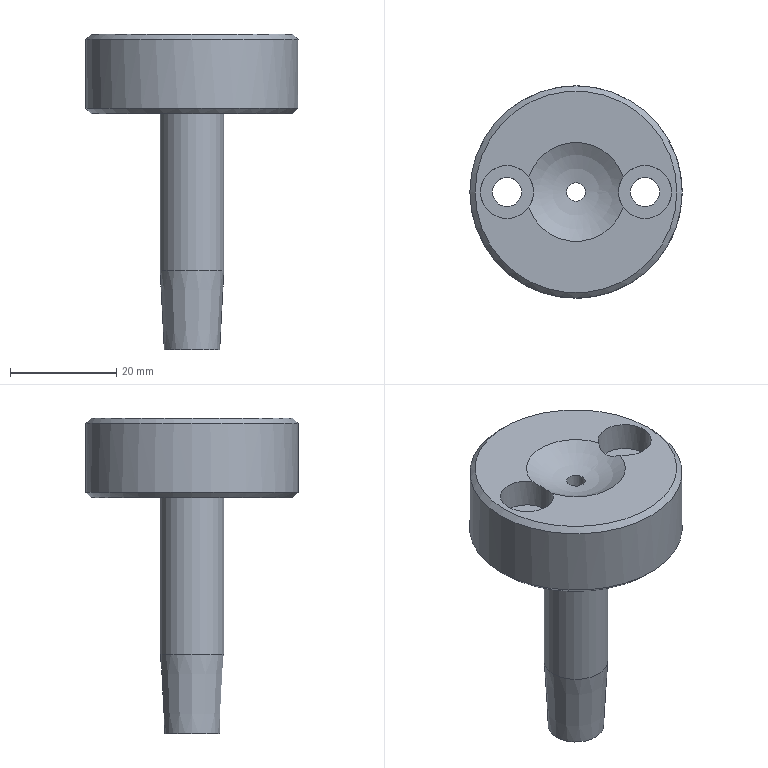Part | STEP file | lll_id154_x_t | 1 solid | 16 faces | box 40 x 40 x 59.5 mm | volume 20901 mm3 | cylinder 6 | plane 5 | cone 4 | sphere 1 | commonest cylinder face diameters 5.5 x2 10 x2 12 x1 40 x1
STEP:
#1=CARTESIAN_POINT('',(-5.214,0.,68.));
#2=VERTEX_POINT('',#1);
#3=CARTESIAN_POINT('',(0.,0.,68.));
#4=DIRECTION('',(0.,0.,1.));
#5=DIRECTION('',(-1.,0.,0.));
#6=AXIS2_PLACEMENT_3D('',#3,#4,#5);
#7=CIRCLE('',#6,5.214);
#8=EDGE_CURVE('',#2,#2,#7,.T.);
#9=ORIENTED_EDGE('',*,*,#8,.F.);
#10=EDGE_LOOP('',(#9));
#11=FACE_BOUND('',#10,.T.);
#12=CARTESIAN_POINT('',(-2.738,0.,68.));
#13=VERTEX_POINT('',#12);
#14=CARTESIAN_POINT('',(0.,0.,68.));
#15=DIRECTION('',(0.,0.,1.));
#16=DIRECTION('',(-1.,0.,0.));
#17=AXIS2_PLACEMENT_3D('',#14,#15,#16);
#18=CIRCLE('',#17,2.738);
#19=EDGE_CURVE('',#13,#13,#18,.T.);
#20=ORIENTED_EDGE('',*,*,#19,.T.);
#21=EDGE_LOOP('',(#20));
#22=FACE_BOUND('',#21,.T.);
#23=CARTESIAN_POINT('',(0.,0.,68.));
#24=DIRECTION('',(0.,0.,-1.));
#25=DIRECTION('',(-1.,0.,0.));
#26=AXIS2_PLACEMENT_3D('',#23,#24,#25);
#27=PLANE('',#26);
#28=ADVANCED_FACE('',(#11,#22),#27,.T.);
#29=CARTESIAN_POINT('',(-19.,0.,112.5));
#30=VERTEX_POINT('',#29);
#31=CARTESIAN_POINT('',(0.,0.,112.5));
#32=DIRECTION('',(0.,0.,-1.));
#33=DIRECTION('',(-1.,0.,0.));
#34=AXIS2_PLACEMENT_3D('',#31,#32,#33);
#35=CIRCLE('',#34,19.);
#36=EDGE_CURVE('',#30,#30,#35,.T.);
#37=ORIENTED_EDGE('',*,*,#36,.T.);
#38=EDGE_LOOP('',(#37));
#39=FACE_BOUND('',#38,.T.);
#40=CARTESIAN_POINT('',(-15.75,0.,112.5));
#41=VERTEX_POINT('',#40);
#42=CARTESIAN_POINT('',(-13.,0.,112.5));
#43=DIRECTION('',(0.,0.,-1.));
#44=DIRECTION('',(-1.,0.,0.));
#45=AXIS2_PLACEMENT_3D('',#42,#43,#44);
#46=CIRCLE('',#45,2.75);
#47=EDGE_CURVE('',#41,#41,#46,.T.);
#48=ORIENTED_EDGE('',*,*,#47,.F.);
#49=EDGE_LOOP('',(#48));
#50=FACE_BOUND('',#49,.T.);
#51=CARTESIAN_POINT('',(10.25,0.,112.5));
#52=VERTEX_POINT('',#51);
#53=CARTESIAN_POINT('',(13.,0.,112.5));
#54=DIRECTION('',(0.,0.,-1.));
#55=DIRECTION('',(-1.,0.,0.));
#56=AXIS2_PLACEMENT_3D('',#53,#54,#55);
#57=CIRCLE('',#56,2.75);
#58=EDGE_CURVE('',#52,#52,#57,.T.);
#59=ORIENTED_EDGE('',*,*,#58,.F.);
#60=EDGE_LOOP('',(#59));
#61=FACE_BOUND('',#60,.T.);
#62=CARTESIAN_POINT('',(-6.,0.,112.5));
#63=VERTEX_POINT('',#62);
#64=CARTESIAN_POINT('',(0.,0.,112.5));
#65=DIRECTION('',(0.,0.,-1.));
#66=DIRECTION('',(-1.,0.,0.));
#67=AXIS2_PLACEMENT_3D('',#64,#65,#66);
#68=CIRCLE('',#67,6.);
#69=EDGE_CURVE('',#63,#63,#68,.T.);
#70=ORIENTED_EDGE('',*,*,#69,.F.);
#71=EDGE_LOOP('',(#70));
#72=FACE_BOUND('',#71,.T.);
#73=CARTESIAN_POINT('',(0.,0.,112.5));
#74=DIRECTION('',(0.,0.,-1.));
#75=DIRECTION('',(-1.,0.,0.));
#76=AXIS2_PLACEMENT_3D('',#73,#74,#75);
#77=PLANE('',#76);
#78=ADVANCED_FACE('',(#39,#50,#61,#72),#77,.T.);
#79=CARTESIAN_POINT('',(19.,0.,127.5));
#80=VERTEX_POINT('',#79);
#81=CARTESIAN_POINT('',(0.,0.,127.5));
#82=DIRECTION('',(0.,0.,1.));
#83=DIRECTION('',(1.,0.,0.));
#84=AXIS2_PLACEMENT_3D('',#81,#82,#83);
#85=CIRCLE('',#84,19.);
#86=EDGE_CURVE('',#80,#80,#85,.T.);
#87=ORIENTED_EDGE('',*,*,#86,.T.);
#88=EDGE_LOOP('',(#87));
#89=FACE_BOUND('',#88,.T.);
#90=CARTESIAN_POINT('',(-8.885,-2.84,127.5));
#91=VERTEX_POINT('',#90);
#92=CARTESIAN_POINT('',(-8.885,2.84,127.5));
#93=VERTEX_POINT('',#92);
#94=CARTESIAN_POINT('',(-13.,0.,127.5));
#95=DIRECTION('',(0.,0.,-1.));
#96=DIRECTION('',(1.,0.,0.));
#97=AXIS2_PLACEMENT_3D('',#94,#95,#96);
#98=CIRCLE('',#97,5.);
#99=EDGE_CURVE('',#91,#93,#98,.T.);
#100=ORIENTED_EDGE('',*,*,#99,.T.);
#101=CARTESIAN_POINT('',(8.885,2.84,127.5));
#102=VERTEX_POINT('',#101);
#103=CARTESIAN_POINT('',(0.,0.,127.5));
#104=DIRECTION('',(0.,0.,1.));
#105=DIRECTION('',(1.,0.,0.));
#106=AXIS2_PLACEMENT_3D('',#103,#104,#105);
#107=CIRCLE('',#106,9.327);
#108=EDGE_CURVE('',#102,#93,#107,.T.);
#109=ORIENTED_EDGE('',*,*,#108,.F.);
#110=CARTESIAN_POINT('',(8.885,-2.84,127.5));
#111=VERTEX_POINT('',#110);
#112=CARTESIAN_POINT('',(13.,0.,127.5));
#113=DIRECTION('',(0.,0.,-1.));
#114=DIRECTION('',(-1.,0.,0.));
#115=AXIS2_PLACEMENT_3D('',#112,#113,#114);
#116=CIRCLE('',#115,5.);
#117=EDGE_CURVE('',#102,#111,#116,.T.);
#118=ORIENTED_EDGE('',*,*,#117,.T.);
#119=CARTESIAN_POINT('',(0.,0.,127.5));
#120=DIRECTION('',(0.,0.,1.));
#121=DIRECTION('',(1.,0.,0.));
#122=AXIS2_PLACEMENT_3D('',#119,#120,#121);
#123=CIRCLE('',#122,9.327);
#124=EDGE_CURVE('',#91,#111,#123,.T.);
#125=ORIENTED_EDGE('',*,*,#124,.F.);
#126=EDGE_LOOP('',(#100,#109,#118,#125));
#127=FACE_BOUND('',#126,.T.);
#128=CARTESIAN_POINT('',(0.,0.,127.5));
#129=DIRECTION('',(0.,0.,1.));
#130=DIRECTION('',(1.,0.,0.));
#131=AXIS2_PLACEMENT_3D('',#128,#129,#130);
#132=PLANE('',#131);
#133=ADVANCED_FACE('',(#89,#127),#132,.T.);
#134=CARTESIAN_POINT('',(-20.,0.,113.5));
#135=VERTEX_POINT('',#134);
#136=CARTESIAN_POINT('',(0.,0.,113.5));
#137=DIRECTION('',(0.,0.,1.));
#138=DIRECTION('',(-1.,0.,0.));
#139=AXIS2_PLACEMENT_3D('',#136,#137,#138);
#140=CIRCLE('',#139,20.);
#141=EDGE_CURVE('',#135,#135,#140,.T.);
#142=ORIENTED_EDGE('',*,*,#141,.T.);
#143=EDGE_LOOP('',(#142));
#144=FACE_BOUND('',#143,.T.);
#145=CARTESIAN_POINT('',(20.,0.,126.5));
#146=VERTEX_POINT('',#145);
#147=CARTESIAN_POINT('',(0.,0.,126.5));
#148=DIRECTION('',(0.,0.,-1.));
#149=DIRECTION('',(1.,0.,0.));
#150=AXIS2_PLACEMENT_3D('',#147,#148,#149);
#151=CIRCLE('',#150,20.);
#152=EDGE_CURVE('',#146,#146,#151,.T.);
#153=ORIENTED_EDGE('',*,*,#152,.T.);
#154=EDGE_LOOP('',(#153));
#155=FACE_BOUND('',#154,.T.);
#156=CARTESIAN_POINT('',(0.,0.,127.5));
#157=DIRECTION('',(0.,0.,-1.));
#158=DIRECTION('',(-1.,0.,0.));
#159=AXIS2_PLACEMENT_3D('',#156,#157,#158);
#160=CYLINDRICAL_SURFACE('',#159,20.);
#161=ADVANCED_FACE('',(#144,#155),#160,.T.);
#162=CARTESIAN_POINT('',(6.,0.,83.));
#163=VERTEX_POINT('',#162);
#164=CARTESIAN_POINT('',(0.,0.,83.));
#165=DIRECTION('',(0.,0.,-1.));
#166=DIRECTION('',(1.,0.,0.));
#167=AXIS2_PLACEMENT_3D('',#164,#165,#166);
#168=CIRCLE('',#167,6.);
#169=EDGE_CURVE('',#163,#163,#168,.T.);
#170=ORIENTED_EDGE('',*,*,#169,.F.);
#171=EDGE_LOOP('',(#170));
#172=FACE_BOUND('',#171,.T.);
#173=ORIENTED_EDGE('',*,*,#69,.T.);
#174=EDGE_LOOP('',(#173));
#175=FACE_BOUND('',#174,.T.);
#176=CARTESIAN_POINT('',(0.,0.,112.5));
#177=DIRECTION('',(0.,0.,-1.));
#178=DIRECTION('',(-1.,0.,0.));
#179=AXIS2_PLACEMENT_3D('',#176,#177,#178);
#180=CYLINDRICAL_SURFACE('',#179,6.);
#181=ADVANCED_FACE('',(#172,#175),#180,.T.);
#182=CARTESIAN_POINT('',(1.75,0.,124.596));
#183=VERTEX_POINT('',#182);
#184=CARTESIAN_POINT('',(0.,0.,124.596));
#185=DIRECTION('',(0.,0.,-1.));
#186=DIRECTION('',(1.,0.,0.));
#187=AXIS2_PLACEMENT_3D('',#184,#185,#186);
#188=CIRCLE('',#187,1.75);
#189=EDGE_CURVE('',#183,#183,#188,.T.);
#190=ORIENTED_EDGE('',*,*,#189,.T.);
#191=EDGE_LOOP('',(#190));
#192=FACE_BOUND('',#191,.T.);
#193=ORIENTED_EDGE('',*,*,#108,.T.);
#194=CARTESIAN_POINT('',(-8.885,2.84,127.5));
#195=CARTESIAN_POINT('',(-8.359,2.077,126.974));
#196=CARTESIAN_POINT('',(-8.001,1.06,126.644));
#197=CARTESIAN_POINT('',(-7.999,-1.053,126.643));
#198=CARTESIAN_POINT('',(-8.358,-2.076,126.973));
#199=CARTESIAN_POINT('',(-8.885,-2.84,127.5));
#200=B_SPLINE_CURVE_WITH_KNOTS('',3,(#194,#195,#196,#197,#198,#199),.UNSPECIFIED.,.F.,.F.,(4,2,4),(0.,0.5,1.),.UNSPECIFIED.);
#201=EDGE_CURVE('',#93,#91,#200,.T.);
#202=ORIENTED_EDGE('',*,*,#201,.T.);
#203=ORIENTED_EDGE('',*,*,#124,.T.);
#204=CARTESIAN_POINT('',(8.885,-2.84,127.5));
#205=CARTESIAN_POINT('',(8.359,-2.077,126.974));
#206=CARTESIAN_POINT('',(8.001,-1.06,126.644));
#207=CARTESIAN_POINT('',(7.999,1.053,126.643));
#208=CARTESIAN_POINT('',(8.358,2.076,126.973));
#209=CARTESIAN_POINT('',(8.885,2.84,127.5));
#210=B_SPLINE_CURVE_WITH_KNOTS('',3,(#204,#205,#206,#207,#208,#209),.UNSPECIFIED.,.F.,.F.,(4,2,4),(0.,0.5,1.),.UNSPECIFIED.);
#211=EDGE_CURVE('',#111,#102,#210,.T.);
#212=ORIENTED_EDGE('',*,*,#211,.T.);
#213=EDGE_LOOP('',(#193,#202,#203,#212));
#214=FACE_BOUND('',#213,.T.);
#215=CARTESIAN_POINT('',(0.,0.,140.5));
#216=DIRECTION('',(0.,0.,1.));
#217=DIRECTION('',(1.,0.,0.));
#218=AXIS2_PLACEMENT_3D('',#215,#216,#217);
#219=SPHERICAL_SURFACE('',#218,16.);
#220=ADVANCED_FACE('',(#192,#214),#219,.F.);
#221=CARTESIAN_POINT('',(8.,0.,122.));
#222=VERTEX_POINT('',#221);
#223=CARTESIAN_POINT('',(13.,0.,122.));
#224=DIRECTION('',(0.,0.,-1.));
#225=DIRECTION('',(-1.,0.,0.));
#226=AXIS2_PLACEMENT_3D('',#223,#224,#225);
#227=CIRCLE('',#226,5.);
#228=EDGE_CURVE('',#222,#222,#227,.T.);
#229=ORIENTED_EDGE('',*,*,#228,.T.);
#230=EDGE_LOOP('',(#229));
#231=FACE_BOUND('',#230,.T.);
#232=ORIENTED_EDGE('',*,*,#117,.F.);
#233=ORIENTED_EDGE('',*,*,#211,.F.);
#234=EDGE_LOOP('',(#232,#233));
#235=FACE_BOUND('',#234,.T.);
#236=CARTESIAN_POINT('',(13.,0.,127.5));
#237=DIRECTION('',(0.,0.,-1.));
#238=DIRECTION('',(-1.,0.,0.));
#239=AXIS2_PLACEMENT_3D('',#236,#237,#238);
#240=CYLINDRICAL_SURFACE('',#239,5.);
#241=ADVANCED_FACE('',(#231,#235),#240,.F.);
#242=ORIENTED_EDGE('',*,*,#58,.T.);
#243=EDGE_LOOP('',(#242));
#244=FACE_BOUND('',#243,.T.);
#245=CARTESIAN_POINT('',(10.25,0.,122.));
#246=VERTEX_POINT('',#245);
#247=CARTESIAN_POINT('',(13.,0.,122.));
#248=DIRECTION('',(0.,0.,-1.));
#249=DIRECTION('',(-1.,0.,0.));
#250=AXIS2_PLACEMENT_3D('',#247,#248,#249);
#251=CIRCLE('',#250,2.75);
#252=EDGE_CURVE('',#246,#246,#251,.T.);
#253=ORIENTED_EDGE('',*,*,#252,.F.);
#254=EDGE_LOOP('',(#253));
#255=FACE_BOUND('',#254,.T.);
#256=CARTESIAN_POINT('',(13.,0.,-172.5));
#257=DIRECTION('',(0.,0.,-1.));
#258=DIRECTION('',(-1.,0.,0.));
#259=AXIS2_PLACEMENT_3D('',#256,#257,#258);
#260=CYLINDRICAL_SURFACE('',#259,2.75);
#261=ADVANCED_FACE('',(#244,#255),#260,.F.);
#262=ORIENTED_EDGE('',*,*,#252,.T.);
#263=EDGE_LOOP('',(#262));
#264=FACE_BOUND('',#263,.T.);
#265=ORIENTED_EDGE('',*,*,#228,.F.);
#266=EDGE_LOOP('',(#265));
#267=FACE_BOUND('',#266,.T.);
#268=CARTESIAN_POINT('',(13.,0.,122.));
#269=DIRECTION('',(0.,0.,-1.));
#270=DIRECTION('',(-1.,0.,0.));
#271=AXIS2_PLACEMENT_3D('',#268,#269,#270);
#272=PLANE('',#271);
#273=ADVANCED_FACE('',(#264,#267),#272,.F.);
#274=CARTESIAN_POINT('',(-8.,0.,122.));
#275=VERTEX_POINT('',#274);
#276=CARTESIAN_POINT('',(-13.,0.,122.));
#277=DIRECTION('',(0.,0.,-1.));
#278=DIRECTION('',(1.,0.,0.));
#279=AXIS2_PLACEMENT_3D('',#276,#277,#278);
#280=CIRCLE('',#279,5.);
#281=EDGE_CURVE('',#275,#275,#280,.T.);
#282=ORIENTED_EDGE('',*,*,#281,.T.);
#283=EDGE_LOOP('',(#282));
#284=FACE_BOUND('',#283,.T.);
#285=ORIENTED_EDGE('',*,*,#99,.F.);
#286=ORIENTED_EDGE('',*,*,#201,.F.);
#287=EDGE_LOOP('',(#285,#286));
#288=FACE_BOUND('',#287,.T.);
#289=CARTESIAN_POINT('',(-13.,0.,127.5));
#290=DIRECTION('',(0.,0.,-1.));
#291=DIRECTION('',(1.,0.,0.));
#292=AXIS2_PLACEMENT_3D('',#289,#290,#291);
#293=CYLINDRICAL_SURFACE('',#292,5.);
#294=ADVANCED_FACE('',(#284,#288),#293,.F.);
#295=ORIENTED_EDGE('',*,*,#47,.T.);
#296=EDGE_LOOP('',(#295));
#297=FACE_BOUND('',#296,.T.);
#298=CARTESIAN_POINT('',(-10.25,0.,122.));
#299=VERTEX_POINT('',#298);
#300=CARTESIAN_POINT('',(-13.,0.,122.));
#301=DIRECTION('',(0.,0.,-1.));
#302=DIRECTION('',(1.,0.,0.));
#303=AXIS2_PLACEMENT_3D('',#300,#301,#302);
#304=CIRCLE('',#303,2.75);
#305=EDGE_CURVE('',#299,#299,#304,.T.);
#306=ORIENTED_EDGE('',*,*,#305,.F.);
#307=EDGE_LOOP('',(#306));
#308=FACE_BOUND('',#307,.T.);
#309=CARTESIAN_POINT('',(-13.,0.,-172.5));
#310=DIRECTION('',(0.,0.,-1.));
#311=DIRECTION('',(1.,0.,0.));
#312=AXIS2_PLACEMENT_3D('',#309,#310,#311);
#313=CYLINDRICAL_SURFACE('',#312,2.75);
#314=ADVANCED_FACE('',(#297,#308),#313,.F.);
#315=ORIENTED_EDGE('',*,*,#305,.T.);
#316=EDGE_LOOP('',(#315));
#317=FACE_BOUND('',#316,.T.);
#318=ORIENTED_EDGE('',*,*,#281,.F.);
#319=EDGE_LOOP('',(#318));
#320=FACE_BOUND('',#319,.T.);
#321=CARTESIAN_POINT('',(-13.,0.,122.));
#322=DIRECTION('',(0.,0.,-1.));
#323=DIRECTION('',(1.,0.,0.));
#324=AXIS2_PLACEMENT_3D('',#321,#322,#323);
#325=PLANE('',#324);
#326=ADVANCED_FACE('',(#317,#320),#325,.F.);
#327=ORIENTED_EDGE('',*,*,#189,.F.);
#328=EDGE_LOOP('',(#327));
#329=FACE_BOUND('',#328,.T.);
#330=ORIENTED_EDGE('',*,*,#19,.F.);
#331=EDGE_LOOP('',(#330));
#332=FACE_BOUND('',#331,.T.);
#333=CARTESIAN_POINT('',(0.,0.,124.596));
#334=DIRECTION('',(0.,0.,-1.));
#335=DIRECTION('',(1.,0.,0.));
#336=AXIS2_PLACEMENT_3D('',#333,#334,#335);
#337=CONICAL_SURFACE('',#336,1.75,1.);
#338=ADVANCED_FACE('',(#329,#332),#337,.F.);
#339=ORIENTED_EDGE('',*,*,#36,.F.);
#340=EDGE_LOOP('',(#339));
#341=FACE_BOUND('',#340,.T.);
#342=ORIENTED_EDGE('',*,*,#141,.F.);
#343=EDGE_LOOP('',(#342));
#344=FACE_BOUND('',#343,.T.);
#345=CARTESIAN_POINT('',(0.,0.,113.5));
#346=DIRECTION('',(0.,0.,1.));
#347=DIRECTION('',(1.,0.,0.));
#348=AXIS2_PLACEMENT_3D('',#345,#346,#347);
#349=CONICAL_SURFACE('',#348,20.,45.);
#350=ADVANCED_FACE('',(#341,#344),#349,.T.);
#351=ORIENTED_EDGE('',*,*,#86,.F.);
#352=EDGE_LOOP('',(#351));
#353=FACE_BOUND('',#352,.T.);
#354=ORIENTED_EDGE('',*,*,#152,.F.);
#355=EDGE_LOOP('',(#354));
#356=FACE_BOUND('',#355,.T.);
#357=CARTESIAN_POINT('',(0.,0.,126.5));
#358=DIRECTION('',(0.,0.,-1.));
#359=DIRECTION('',(-1.,0.,0.));
#360=AXIS2_PLACEMENT_3D('',#357,#358,#359);
#361=CONICAL_SURFACE('',#360,20.,45.);
#362=ADVANCED_FACE('',(#353,#356),#361,.T.);
#363=ORIENTED_EDGE('',*,*,#8,.T.);
#364=EDGE_LOOP('',(#363));
#365=FACE_BOUND('',#364,.T.);
#366=ORIENTED_EDGE('',*,*,#169,.T.);
#367=EDGE_LOOP('',(#366));
#368=FACE_BOUND('',#367,.T.);
#369=CARTESIAN_POINT('',(0.,0.,83.));
#370=DIRECTION('',(0.,0.,1.));
#371=DIRECTION('',(1.,0.,0.));
#372=AXIS2_PLACEMENT_3D('',#369,#370,#371);
#373=CONICAL_SURFACE('',#372,6.,3.);
#374=ADVANCED_FACE('',(#365,#368),#373,.T.);
#375=CLOSED_SHELL('',(#28,#78,#133,#161,#181,#220,#241,#261,#273,#294,#314,#326,#338,#350,#362,#374));
#376=MANIFOLD_SOLID_BREP('',#375);
#377=(LENGTH_UNIT()NAMED_UNIT(*)SI_UNIT(.MILLI.,.METRE.));
#378=UNCERTAINTY_MEASURE_WITH_UNIT(LENGTH_MEASURE(0.0508),#377,'','');
#379=(NAMED_UNIT(*)PLANE_ANGLE_UNIT()SI_UNIT($,.RADIAN.));
#380=PLANE_ANGLE_MEASURE_WITH_UNIT(PLANE_ANGLE_MEASURE(0.01745),#379);
#381=DIMENSIONAL_EXPONENTS(0.,0.,0.,0.,0.,0.,0.);
#382=(CONVERSION_BASED_UNIT('DEGREE',#380)NAMED_UNIT(#381)PLANE_ANGLE_UNIT());
#383=(NAMED_UNIT(*)SI_UNIT($,.STERADIAN.)SOLID_ANGLE_UNIT());
#384=(GEOMETRIC_REPRESENTATION_CONTEXT(3)GLOBAL_UNCERTAINTY_ASSIGNED_CONTEXT((#378))GLOBAL_UNIT_ASSIGNED_CONTEXT((#377,#382,#383))REPRESENTATION_CONTEXT('',''));
#385=ADVANCED_BREP_SHAPE_REPRESENTATION('',(#376),#384);